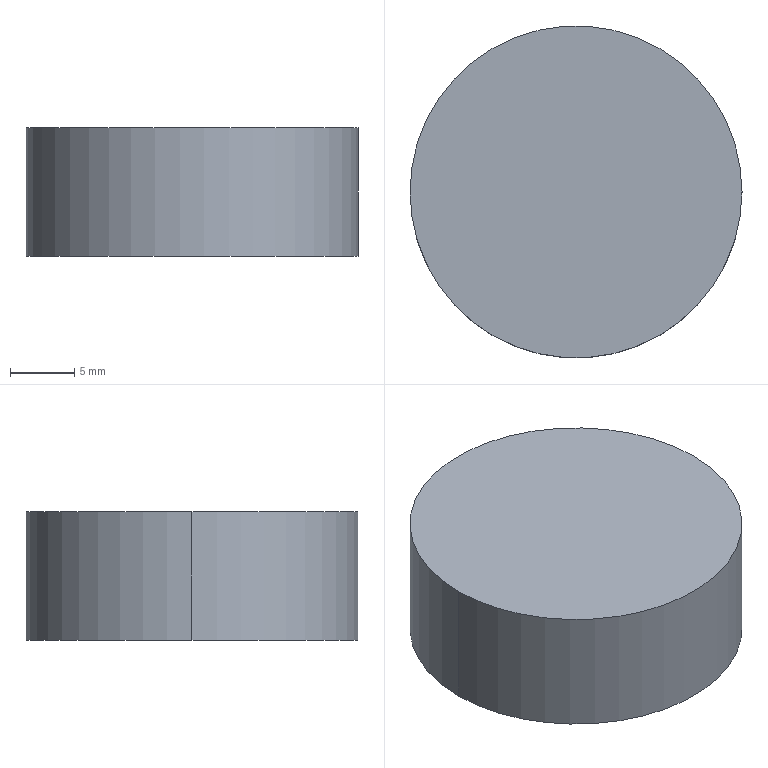Part | SolidWorks | features Extrusion 1 | 1 solid | 4 faces | box 25.927 x 25.927 x 10 mm | volume 5280 mm3 | cylinder 2 | plane 2 | commonest cylinder face diameters 25.927 x2
STEP:
#1=CARTESIAN_POINT('',(-4.092,0.,10.));
#2=VERTEX_POINT('',#1);
#3=CARTESIAN_POINT('',(-30.019,0.,10.));
#4=VERTEX_POINT('',#3);
#5=CARTESIAN_POINT('',(-17.056,0.,10.));
#6=DIRECTION('',(0.,0.,1.));
#7=DIRECTION('',(1.,0.,0.));
#8=AXIS2_PLACEMENT_3D('',#5,#6,#7);
#9=CIRCLE('',#8,12.964);
#10=EDGE_CURVE('',#2,#4,#9,.T.);
#11=ORIENTED_EDGE('',*,*,#10,.F.);
#12=CARTESIAN_POINT('',(-4.092,0.,0.));
#13=VERTEX_POINT('',#12);
#14=CARTESIAN_POINT('',(-4.092,0.,10.));
#15=DIRECTION('',(0.,0.,-1.));
#16=VECTOR('',#15,1000.);
#17=LINE('',#14,#16);
#18=EDGE_CURVE('',#2,#13,#17,.T.);
#19=ORIENTED_EDGE('',*,*,#18,.T.);
#20=CARTESIAN_POINT('',(-30.019,0.,0.));
#21=VERTEX_POINT('',#20);
#22=CARTESIAN_POINT('',(-17.056,0.,0.));
#23=DIRECTION('',(0.,0.,1.));
#24=DIRECTION('',(1.,0.,0.));
#25=AXIS2_PLACEMENT_3D('',#22,#23,#24);
#26=CIRCLE('',#25,12.964);
#27=EDGE_CURVE('',#13,#21,#26,.T.);
#28=ORIENTED_EDGE('',*,*,#27,.T.);
#29=CARTESIAN_POINT('',(-30.019,0.,10.));
#30=DIRECTION('',(0.,0.,-1.));
#31=VECTOR('',#30,1000.);
#32=LINE('',#29,#31);
#33=EDGE_CURVE('',#4,#21,#32,.T.);
#34=ORIENTED_EDGE('',*,*,#33,.F.);
#35=EDGE_LOOP('',(#11,#19,#28,#34));
#36=FACE_OUTER_BOUND('',#35,.T.);
#37=CARTESIAN_POINT('',(-17.056,0.,10.));
#38=DIRECTION('',(0.,0.,-1.));
#39=DIRECTION('',(-1.,0.,0.));
#40=AXIS2_PLACEMENT_3D('',#37,#38,#39);
#41=CYLINDRICAL_SURFACE('',#40,12.964);
#42=ADVANCED_FACE('',(#36),#41,.T.);
#43=ORIENTED_EDGE('',*,*,#18,.F.);
#44=CARTESIAN_POINT('',(-17.056,0.,10.));
#45=DIRECTION('',(0.,0.,1.));
#46=DIRECTION('',(1.,0.,0.));
#47=AXIS2_PLACEMENT_3D('',#44,#45,#46);
#48=CIRCLE('',#47,12.964);
#49=EDGE_CURVE('',#4,#2,#48,.T.);
#50=ORIENTED_EDGE('',*,*,#49,.F.);
#51=ORIENTED_EDGE('',*,*,#33,.T.);
#52=CARTESIAN_POINT('',(-17.056,0.,0.));
#53=DIRECTION('',(0.,0.,1.));
#54=DIRECTION('',(1.,0.,0.));
#55=AXIS2_PLACEMENT_3D('',#52,#53,#54);
#56=CIRCLE('',#55,12.964);
#57=EDGE_CURVE('',#21,#13,#56,.T.);
#58=ORIENTED_EDGE('',*,*,#57,.T.);
#59=EDGE_LOOP('',(#43,#50,#51,#58));
#60=FACE_OUTER_BOUND('',#59,.T.);
#61=CARTESIAN_POINT('',(-17.056,0.,10.));
#62=DIRECTION('',(0.,0.,-1.));
#63=DIRECTION('',(-1.,0.,0.));
#64=AXIS2_PLACEMENT_3D('',#61,#62,#63);
#65=CYLINDRICAL_SURFACE('',#64,12.964);
#66=ADVANCED_FACE('',(#60),#65,.T.);
#67=ORIENTED_EDGE('',*,*,#49,.T.);
#68=ORIENTED_EDGE('',*,*,#10,.T.);
#69=EDGE_LOOP('',(#67,#68));
#70=FACE_OUTER_BOUND('',#69,.T.);
#71=CARTESIAN_POINT('',(-17.056,0.,10.));
#72=DIRECTION('',(0.,0.,1.));
#73=DIRECTION('',(1.,0.,0.));
#74=AXIS2_PLACEMENT_3D('',#71,#72,#73);
#75=PLANE('',#74);
#76=ADVANCED_FACE('',(#70),#75,.T.);
#77=ORIENTED_EDGE('',*,*,#57,.F.);
#78=ORIENTED_EDGE('',*,*,#27,.F.);
#79=EDGE_LOOP('',(#77,#78));
#80=FACE_OUTER_BOUND('',#79,.T.);
#81=CARTESIAN_POINT('',(-17.056,0.,0.));
#82=DIRECTION('',(0.,0.,1.));
#83=DIRECTION('',(1.,0.,0.));
#84=AXIS2_PLACEMENT_3D('',#81,#82,#83);
#85=PLANE('',#84);
#86=ADVANCED_FACE('',(#80),#85,.F.);
#87=CLOSED_SHELL('',(#42,#66,#76,#86));
#88=MANIFOLD_SOLID_BREP('',#87);
#89=CARTESIAN_POINT('',(0.,0.,0.));
#90=DIRECTION('',(0.,0.,1.));
#91=DIRECTION('',(1.,0.,0.));
#92=AXIS2_PLACEMENT_3D('',#89,#90,#91);
#93=(LENGTH_UNIT()NAMED_UNIT(*)SI_UNIT(.MILLI.,.METRE.));
#94=UNCERTAINTY_MEASURE_WITH_UNIT(LENGTH_MEASURE(0.00001),#93,'','');
#95=(NAMED_UNIT(*)PLANE_ANGLE_UNIT()SI_UNIT($,.RADIAN.));
#96=(NAMED_UNIT(*)SI_UNIT($,.STERADIAN.)SOLID_ANGLE_UNIT());
#97=(GEOMETRIC_REPRESENTATION_CONTEXT(3)GLOBAL_UNCERTAINTY_ASSIGNED_CONTEXT((#94))GLOBAL_UNIT_ASSIGNED_CONTEXT((#93,#95,#96))REPRESENTATION_CONTEXT('',''));
#98=ADVANCED_BREP_SHAPE_REPRESENTATION('',(#88,#92),#97);